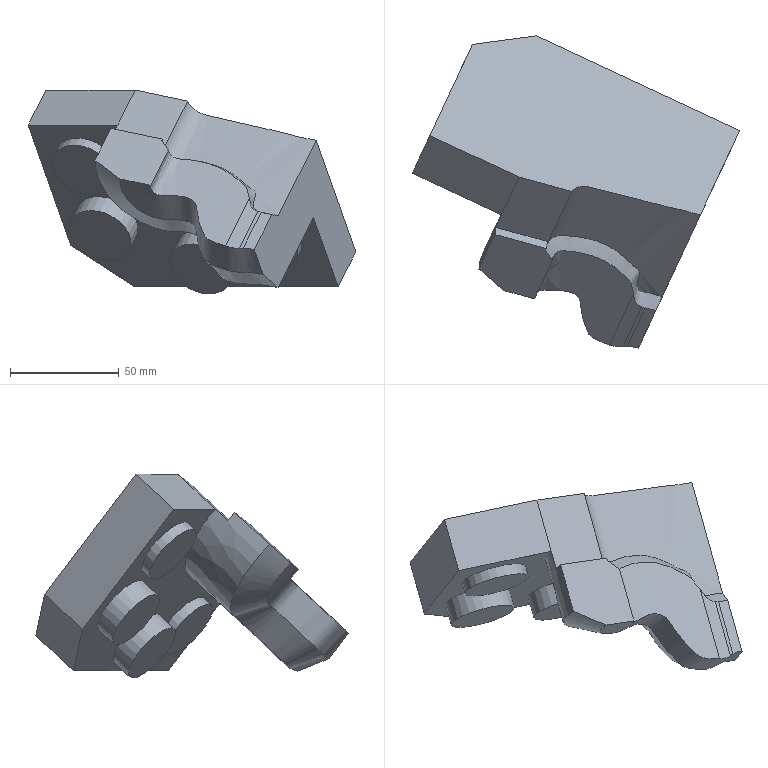Part | NX | features solid 2 | 1 solid | 27 faces | box 150.445 x 143.52 x 93.645 mm | volume 400738 mm3 | plane 15 | spline 8 | cylinder 4 | commonest cylinder face diameters 30 x4